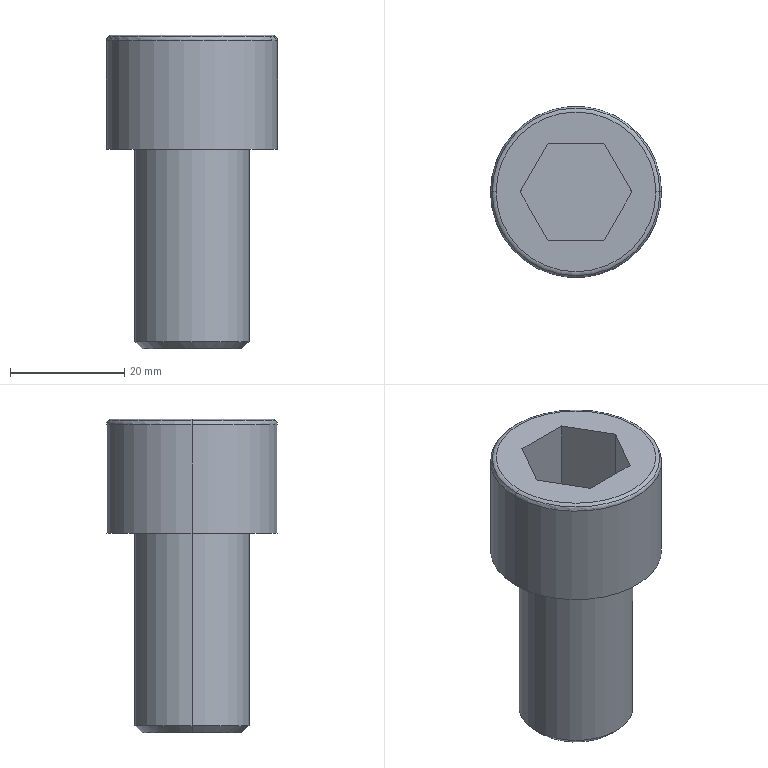Part | Creo | 1 solid | 20 faces | box 30 x 30 x 55 mm | volume 21762 mm3 | plane 10 | cylinder 4 | torus 4 | cone 2 | commonest cylinder face diameters 20 x2 30 x2
STEP:
#1=CARTESIAN_POINT('',(255.,70.,140.75));
#2=VERTEX_POINT('',#1);
#3=CARTESIAN_POINT('',(275.,70.,140.75));
#4=VERTEX_POINT('',#3);
#5=CARTESIAN_POINT('',(265.,70.,140.75));
#6=DIRECTION('',(0.,0.,-1.));
#7=DIRECTION('',(-1.,0.,0.));
#8=AXIS2_PLACEMENT_3D('',#5,#6,#7);
#9=CIRCLE('',#8,10.);
#10=EDGE_CURVE('',#2,#4,#9,.T.);
#11=ORIENTED_EDGE('',*,*,#10,.T.);
#12=CARTESIAN_POINT('',(275.,70.,174.5));
#13=VERTEX_POINT('',#12);
#14=CARTESIAN_POINT('',(275.,70.,174.5));
#15=DIRECTION('',(0.,0.,-1.));
#16=VECTOR('',#15,33.75);
#17=LINE('',#14,#16);
#18=EDGE_CURVE('',#13,#4,#17,.T.);
#19=ORIENTED_EDGE('',*,*,#18,.F.);
#20=CARTESIAN_POINT('',(255.,70.,174.5));
#21=VERTEX_POINT('',#20);
#22=CARTESIAN_POINT('',(265.,70.,174.5));
#23=DIRECTION('',(0.,0.,1.));
#24=DIRECTION('',(1.,0.,0.));
#25=AXIS2_PLACEMENT_3D('',#22,#23,#24);
#26=CIRCLE('',#25,10.);
#27=EDGE_CURVE('',#13,#21,#26,.T.);
#28=ORIENTED_EDGE('',*,*,#27,.T.);
#29=CARTESIAN_POINT('',(255.,70.,174.5));
#30=DIRECTION('',(0.,0.,-1.));
#31=VECTOR('',#30,33.75);
#32=LINE('',#29,#31);
#33=EDGE_CURVE('',#21,#2,#32,.T.);
#34=ORIENTED_EDGE('',*,*,#33,.T.);
#35=EDGE_LOOP('',(#11,#19,#28,#34));
#36=FACE_OUTER_BOUND('',#35,.F.);
#37=CARTESIAN_POINT('',(265.,70.,174.5));
#38=DIRECTION('',(0.,0.,-1.));
#39=DIRECTION('',(-1.,0.,0.));
#40=AXIS2_PLACEMENT_3D('',#37,#38,#39);
#41=CYLINDRICAL_SURFACE('',#40,10.);
#42=ADVANCED_FACE('',(#36),#41,.T.);
#43=CARTESIAN_POINT('',(256.25,70.,139.5));
#44=VERTEX_POINT('',#43);
#45=CARTESIAN_POINT('',(273.75,70.,139.5));
#46=VERTEX_POINT('',#45);
#47=CARTESIAN_POINT('',(265.,70.,139.5));
#48=DIRECTION('',(0.,0.,-1.));
#49=DIRECTION('',(-1.,0.,0.));
#50=AXIS2_PLACEMENT_3D('',#47,#48,#49);
#51=CIRCLE('',#50,8.75);
#52=EDGE_CURVE('',#44,#46,#51,.T.);
#53=ORIENTED_EDGE('',*,*,#52,.T.);
#54=CARTESIAN_POINT('',(273.75,70.,139.5));
#55=DIRECTION('',(0.7071,0.,0.7071));
#56=VECTOR('',#55,1.768);
#57=LINE('',#54,#56);
#58=EDGE_CURVE('',#46,#4,#57,.T.);
#59=ORIENTED_EDGE('',*,*,#58,.T.);
#60=ORIENTED_EDGE('',*,*,#10,.F.);
#61=CARTESIAN_POINT('',(256.25,70.,139.5));
#62=DIRECTION('',(-0.7071,0.,0.7071));
#63=VECTOR('',#62,1.768);
#64=LINE('',#61,#63);
#65=EDGE_CURVE('',#44,#2,#64,.T.);
#66=ORIENTED_EDGE('',*,*,#65,.F.);
#67=EDGE_LOOP('',(#53,#59,#60,#66));
#68=FACE_OUTER_BOUND('',#67,.F.);
#69=CARTESIAN_POINT('',(265.,70.,140.125));
#70=DIRECTION('',(0.,0.,1.));
#71=DIRECTION('',(1.,0.,0.));
#72=AXIS2_PLACEMENT_3D('',#69,#70,#71);
#73=CONICAL_SURFACE('',#72,9.375,45.);
#74=ADVANCED_FACE('',(#68),#73,.T.);
#75=CARTESIAN_POINT('',(265.,70.,139.5));
#76=DIRECTION('',(0.,0.,-1.));
#77=DIRECTION('',(1.,0.,0.));
#78=AXIS2_PLACEMENT_3D('',#75,#76,#77);
#79=CIRCLE('',#78,8.75);
#80=EDGE_CURVE('',#46,#44,#79,.T.);
#81=ORIENTED_EDGE('',*,*,#80,.F.);
#82=ORIENTED_EDGE('',*,*,#52,.F.);
#83=EDGE_LOOP('',(#81,#82));
#84=FACE_OUTER_BOUND('',#83,.F.);
#85=CARTESIAN_POINT('',(265.,70.,139.5));
#86=DIRECTION('',(0.,0.,1.));
#87=DIRECTION('',(1.,0.,0.));
#88=AXIS2_PLACEMENT_3D('',#85,#86,#87);
#89=PLANE('',#88);
#90=ADVANCED_FACE('',(#84),#89,.F.);
#91=ORIENTED_EDGE('',*,*,#80,.T.);
#92=ORIENTED_EDGE('',*,*,#65,.T.);
#93=CARTESIAN_POINT('',(265.,70.,140.75));
#94=DIRECTION('',(0.,0.,-1.));
#95=DIRECTION('',(1.,0.,0.));
#96=AXIS2_PLACEMENT_3D('',#93,#94,#95);
#97=CIRCLE('',#96,10.);
#98=EDGE_CURVE('',#4,#2,#97,.T.);
#99=ORIENTED_EDGE('',*,*,#98,.F.);
#100=ORIENTED_EDGE('',*,*,#58,.F.);
#101=EDGE_LOOP('',(#91,#92,#99,#100));
#102=FACE_OUTER_BOUND('',#101,.F.);
#103=CARTESIAN_POINT('',(265.,70.,140.125));
#104=DIRECTION('',(0.,0.,1.));
#105=DIRECTION('',(1.,0.,0.));
#106=AXIS2_PLACEMENT_3D('',#103,#104,#105);
#107=CONICAL_SURFACE('',#106,9.375,45.);
#108=ADVANCED_FACE('',(#102),#107,.T.);
#109=ORIENTED_EDGE('',*,*,#98,.T.);
#110=ORIENTED_EDGE('',*,*,#33,.F.);
#111=CARTESIAN_POINT('',(265.,70.,174.5));
#112=DIRECTION('',(0.,0.,1.));
#113=DIRECTION('',(-1.,0.,0.));
#114=AXIS2_PLACEMENT_3D('',#111,#112,#113);
#115=CIRCLE('',#114,10.);
#116=EDGE_CURVE('',#21,#13,#115,.T.);
#117=ORIENTED_EDGE('',*,*,#116,.T.);
#118=ORIENTED_EDGE('',*,*,#18,.T.);
#119=EDGE_LOOP('',(#109,#110,#117,#118));
#120=FACE_OUTER_BOUND('',#119,.F.);
#121=CARTESIAN_POINT('',(265.,70.,174.5));
#122=DIRECTION('',(0.,0.,-1.));
#123=DIRECTION('',(-1.,0.,0.));
#124=AXIS2_PLACEMENT_3D('',#121,#122,#123);
#125=CYLINDRICAL_SURFACE('',#124,10.);
#126=ADVANCED_FACE('',(#120),#125,.T.);
#127=CARTESIAN_POINT('',(280.,70.,174.5));
#128=VERTEX_POINT('',#127);
#129=CARTESIAN_POINT('',(250.,70.,174.5));
#130=VERTEX_POINT('',#129);
#131=CARTESIAN_POINT('',(265.,70.,174.5));
#132=DIRECTION('',(0.,0.,-1.));
#133=DIRECTION('',(1.,0.,0.));
#134=AXIS2_PLACEMENT_3D('',#131,#132,#133);
#135=CIRCLE('',#134,15.);
#136=EDGE_CURVE('',#128,#130,#135,.T.);
#137=ORIENTED_EDGE('',*,*,#136,.F.);
#138=CARTESIAN_POINT('',(265.,70.,174.5));
#139=DIRECTION('',(0.,0.,-1.));
#140=DIRECTION('',(-1.,0.,0.));
#141=AXIS2_PLACEMENT_3D('',#138,#139,#140);
#142=CIRCLE('',#141,15.);
#143=EDGE_CURVE('',#130,#128,#142,.T.);
#144=ORIENTED_EDGE('',*,*,#143,.F.);
#145=EDGE_LOOP('',(#137,#144));
#146=FACE_OUTER_BOUND('',#145,.F.);
#147=ORIENTED_EDGE('',*,*,#27,.F.);
#148=ORIENTED_EDGE('',*,*,#116,.F.);
#149=EDGE_LOOP('',(#147,#148));
#150=FACE_BOUND('',#149,.F.);
#151=CARTESIAN_POINT('',(265.,70.,174.5));
#152=DIRECTION('',(0.,0.,-1.));
#153=DIRECTION('',(-1.,0.,0.));
#154=AXIS2_PLACEMENT_3D('',#151,#152,#153);
#155=PLANE('',#154);
#156=ADVANCED_FACE('',(#146,#150),#155,.T.);
#157=CARTESIAN_POINT('',(250.,70.,193.5));
#158=VERTEX_POINT('',#157);
#159=CARTESIAN_POINT('',(280.,70.,193.5));
#160=VERTEX_POINT('',#159);
#161=CARTESIAN_POINT('',(265.,70.,193.5));
#162=DIRECTION('',(0.,0.,1.));
#163=DIRECTION('',(-1.,0.,0.));
#164=AXIS2_PLACEMENT_3D('',#161,#162,#163);
#165=CIRCLE('',#164,15.);
#166=EDGE_CURVE('',#158,#160,#165,.T.);
#167=ORIENTED_EDGE('',*,*,#166,.T.);
#168=CARTESIAN_POINT('',(280.,70.,174.5));
#169=DIRECTION('',(0.,0.,1.));
#170=VECTOR('',#169,19.);
#171=LINE('',#168,#170);
#172=EDGE_CURVE('',#128,#160,#171,.T.);
#173=ORIENTED_EDGE('',*,*,#172,.F.);
#174=ORIENTED_EDGE('',*,*,#136,.T.);
#175=CARTESIAN_POINT('',(250.,70.,174.5));
#176=DIRECTION('',(0.,0.,1.));
#177=VECTOR('',#176,19.);
#178=LINE('',#175,#177);
#179=EDGE_CURVE('',#130,#158,#178,.T.);
#180=ORIENTED_EDGE('',*,*,#179,.T.);
#181=EDGE_LOOP('',(#167,#173,#174,#180));
#182=FACE_OUTER_BOUND('',#181,.F.);
#183=CARTESIAN_POINT('',(265.,70.,174.5));
#184=DIRECTION('',(0.,0.,1.));
#185=DIRECTION('',(1.,0.,0.));
#186=AXIS2_PLACEMENT_3D('',#183,#184,#185);
#187=CYLINDRICAL_SURFACE('',#186,15.);
#188=ADVANCED_FACE('',(#182),#187,.T.);
#189=ORIENTED_EDGE('',*,*,#166,.F.);
#190=CARTESIAN_POINT('',(250.293,70.,194.207));
#191=VERTEX_POINT('',#190);
#192=CARTESIAN_POINT('',(251.,70.,193.5));
#193=DIRECTION('',(0.,1.,0.));
#194=DIRECTION('',(-1.,0.,0.));
#195=AXIS2_PLACEMENT_3D('',#192,#193,#194);
#196=CIRCLE('',#195,1.);
#197=EDGE_CURVE('',#158,#191,#196,.T.);
#198=ORIENTED_EDGE('',*,*,#197,.T.);
#199=CARTESIAN_POINT('',(279.707,70.,194.207));
#200=VERTEX_POINT('',#199);
#201=CARTESIAN_POINT('',(265.,70.,194.207));
#202=DIRECTION('',(0.,0.,1.));
#203=DIRECTION('',(-1.,0.,0.));
#204=AXIS2_PLACEMENT_3D('',#201,#202,#203);
#205=CIRCLE('',#204,14.707);
#206=EDGE_CURVE('',#191,#200,#205,.T.);
#207=ORIENTED_EDGE('',*,*,#206,.T.);
#208=CARTESIAN_POINT('',(279.,70.,193.5));
#209=DIRECTION('',(0.,-1.,0.));
#210=DIRECTION('',(1.,0.,0.));
#211=AXIS2_PLACEMENT_3D('',#208,#209,#210);
#212=CIRCLE('',#211,1.);
#213=EDGE_CURVE('',#160,#200,#212,.T.);
#214=ORIENTED_EDGE('',*,*,#213,.F.);
#215=EDGE_LOOP('',(#189,#198,#207,#214));
#216=FACE_OUTER_BOUND('',#215,.F.);
#217=CARTESIAN_POINT('',(265.,70.,193.5));
#218=DIRECTION('',(0.,0.,1.));
#219=DIRECTION('',(1.,0.,0.));
#220=AXIS2_PLACEMENT_3D('',#217,#218,#219);
#221=TOROIDAL_SURFACE('',#220,14.,1.);
#222=ADVANCED_FACE('',(#216),#221,.T.);
#223=CARTESIAN_POINT('',(265.,70.,193.5));
#224=DIRECTION('',(0.,0.,1.));
#225=DIRECTION('',(1.,0.,0.));
#226=AXIS2_PLACEMENT_3D('',#223,#224,#225);
#227=CIRCLE('',#226,15.);
#228=EDGE_CURVE('',#160,#158,#227,.T.);
#229=ORIENTED_EDGE('',*,*,#228,.F.);
#230=ORIENTED_EDGE('',*,*,#213,.T.);
#231=CARTESIAN_POINT('',(265.,70.,194.207));
#232=DIRECTION('',(0.,0.,1.));
#233=DIRECTION('',(1.,0.,0.));
#234=AXIS2_PLACEMENT_3D('',#231,#232,#233);
#235=CIRCLE('',#234,14.707);
#236=EDGE_CURVE('',#200,#191,#235,.T.);
#237=ORIENTED_EDGE('',*,*,#236,.T.);
#238=ORIENTED_EDGE('',*,*,#197,.F.);
#239=EDGE_LOOP('',(#229,#230,#237,#238));
#240=FACE_OUTER_BOUND('',#239,.F.);
#241=CARTESIAN_POINT('',(265.,70.,193.5));
#242=DIRECTION('',(0.,0.,1.));
#243=DIRECTION('',(1.,0.,0.));
#244=AXIS2_PLACEMENT_3D('',#241,#242,#243);
#245=TOROIDAL_SURFACE('',#244,14.,1.);
#246=ADVANCED_FACE('',(#240),#245,.T.);
#247=ORIENTED_EDGE('',*,*,#228,.T.);
#248=ORIENTED_EDGE('',*,*,#179,.F.);
#249=ORIENTED_EDGE('',*,*,#143,.T.);
#250=ORIENTED_EDGE('',*,*,#172,.T.);
#251=EDGE_LOOP('',(#247,#248,#249,#250));
#252=FACE_OUTER_BOUND('',#251,.F.);
#253=CARTESIAN_POINT('',(265.,70.,174.5));
#254=DIRECTION('',(0.,0.,1.));
#255=DIRECTION('',(1.,0.,0.));
#256=AXIS2_PLACEMENT_3D('',#253,#254,#255);
#257=CYLINDRICAL_SURFACE('',#256,15.);
#258=ADVANCED_FACE('',(#252),#257,.T.);
#259=CARTESIAN_POINT('',(279.,70.,194.5));
#260=VERTEX_POINT('',#259);
#261=CARTESIAN_POINT('',(251.,70.,194.5));
#262=VERTEX_POINT('',#261);
#263=CARTESIAN_POINT('',(265.,70.,194.5));
#264=DIRECTION('',(0.,0.,1.));
#265=DIRECTION('',(1.,0.,0.));
#266=AXIS2_PLACEMENT_3D('',#263,#264,#265);
#267=CIRCLE('',#266,14.);
#268=EDGE_CURVE('',#260,#262,#267,.T.);
#269=ORIENTED_EDGE('',*,*,#268,.T.);
#270=CARTESIAN_POINT('',(251.,70.,193.5));
#271=DIRECTION('',(0.,1.,0.));
#272=DIRECTION('',(-0.7071,0.,0.7071));
#273=AXIS2_PLACEMENT_3D('',#270,#271,#272);
#274=CIRCLE('',#273,1.);
#275=EDGE_CURVE('',#191,#262,#274,.T.);
#276=ORIENTED_EDGE('',*,*,#275,.F.);
#277=ORIENTED_EDGE('',*,*,#236,.F.);
#278=CARTESIAN_POINT('',(279.,70.,193.5));
#279=DIRECTION('',(0.,-1.,0.));
#280=DIRECTION('',(0.7071,0.,0.7071));
#281=AXIS2_PLACEMENT_3D('',#278,#279,#280);
#282=CIRCLE('',#281,1.);
#283=EDGE_CURVE('',#200,#260,#282,.T.);
#284=ORIENTED_EDGE('',*,*,#283,.T.);
#285=EDGE_LOOP('',(#269,#276,#277,#284));
#286=FACE_OUTER_BOUND('',#285,.F.);
#287=CARTESIAN_POINT('',(265.,70.,193.5));
#288=DIRECTION('',(0.,0.,1.));
#289=DIRECTION('',(1.,0.,0.));
#290=AXIS2_PLACEMENT_3D('',#287,#288,#289);
#291=TOROIDAL_SURFACE('',#290,14.,1.);
#292=ADVANCED_FACE('',(#286),#291,.T.);
#293=ORIENTED_EDGE('',*,*,#268,.F.);
#294=CARTESIAN_POINT('',(265.,70.,194.5));
#295=DIRECTION('',(0.,0.,1.));
#296=DIRECTION('',(-1.,0.,0.));
#297=AXIS2_PLACEMENT_3D('',#294,#295,#296);
#298=CIRCLE('',#297,14.);
#299=EDGE_CURVE('',#262,#260,#298,.T.);
#300=ORIENTED_EDGE('',*,*,#299,.F.);
#301=EDGE_LOOP('',(#293,#300));
#302=FACE_OUTER_BOUND('',#301,.F.);
#303=CARTESIAN_POINT('',(269.907,61.5,194.5));
#304=VERTEX_POINT('',#303);
#305=CARTESIAN_POINT('',(260.093,61.5,194.5));
#306=VERTEX_POINT('',#305);
#307=CARTESIAN_POINT('',(269.907,61.5,194.5));
#308=DIRECTION('',(-1.,0.,0.));
#309=VECTOR('',#308,9.815);
#310=LINE('',#307,#309);
#311=EDGE_CURVE('',#304,#306,#310,.T.);
#312=ORIENTED_EDGE('',*,*,#311,.F.);
#313=CARTESIAN_POINT('',(274.815,70.,194.5));
#314=VERTEX_POINT('',#313);
#315=CARTESIAN_POINT('',(274.815,70.,194.5));
#316=DIRECTION('',(-0.5,-0.866,0.));
#317=VECTOR('',#316,9.815);
#318=LINE('',#315,#317);
#319=EDGE_CURVE('',#314,#304,#318,.T.);
#320=ORIENTED_EDGE('',*,*,#319,.F.);
#321=CARTESIAN_POINT('',(269.907,78.5,194.5));
#322=VERTEX_POINT('',#321);
#323=CARTESIAN_POINT('',(269.907,78.5,194.5));
#324=DIRECTION('',(0.5,-0.866,0.));
#325=VECTOR('',#324,9.815);
#326=LINE('',#323,#325);
#327=EDGE_CURVE('',#322,#314,#326,.T.);
#328=ORIENTED_EDGE('',*,*,#327,.F.);
#329=CARTESIAN_POINT('',(260.093,78.5,194.5));
#330=VERTEX_POINT('',#329);
#331=CARTESIAN_POINT('',(260.093,78.5,194.5));
#332=DIRECTION('',(1.,0.,0.));
#333=VECTOR('',#332,9.815);
#334=LINE('',#331,#333);
#335=EDGE_CURVE('',#330,#322,#334,.T.);
#336=ORIENTED_EDGE('',*,*,#335,.F.);
#337=CARTESIAN_POINT('',(255.185,70.,194.5));
#338=VERTEX_POINT('',#337);
#339=CARTESIAN_POINT('',(255.185,70.,194.5));
#340=DIRECTION('',(0.5,0.866,0.));
#341=VECTOR('',#340,9.815);
#342=LINE('',#339,#341);
#343=EDGE_CURVE('',#338,#330,#342,.T.);
#344=ORIENTED_EDGE('',*,*,#343,.F.);
#345=CARTESIAN_POINT('',(260.093,61.5,194.5));
#346=DIRECTION('',(-0.5,0.866,0.));
#347=VECTOR('',#346,9.815);
#348=LINE('',#345,#347);
#349=EDGE_CURVE('',#306,#338,#348,.T.);
#350=ORIENTED_EDGE('',*,*,#349,.F.);
#351=EDGE_LOOP('',(#312,#320,#328,#336,#344,#350));
#352=FACE_BOUND('',#351,.F.);
#353=CARTESIAN_POINT('',(265.,70.,194.5));
#354=DIRECTION('',(0.,0.,1.));
#355=DIRECTION('',(1.,0.,0.));
#356=AXIS2_PLACEMENT_3D('',#353,#354,#355);
#357=PLANE('',#356);
#358=ADVANCED_FACE('',(#302,#352),#357,.T.);
#359=ORIENTED_EDGE('',*,*,#299,.T.);
#360=ORIENTED_EDGE('',*,*,#283,.F.);
#361=ORIENTED_EDGE('',*,*,#206,.F.);
#362=ORIENTED_EDGE('',*,*,#275,.T.);
#363=EDGE_LOOP('',(#359,#360,#361,#362));
#364=FACE_OUTER_BOUND('',#363,.F.);
#365=CARTESIAN_POINT('',(265.,70.,193.5));
#366=DIRECTION('',(0.,0.,1.));
#367=DIRECTION('',(1.,0.,0.));
#368=AXIS2_PLACEMENT_3D('',#365,#366,#367);
#369=TOROIDAL_SURFACE('',#368,14.,1.);
#370=ADVANCED_FACE('',(#364),#369,.T.);
#371=ORIENTED_EDGE('',*,*,#311,.T.);
#372=CARTESIAN_POINT('',(260.093,61.5,181.3));
#373=VERTEX_POINT('',#372);
#374=CARTESIAN_POINT('',(260.093,61.5,194.5));
#375=DIRECTION('',(0.,0.,-1.));
#376=VECTOR('',#375,13.2);
#377=LINE('',#374,#376);
#378=EDGE_CURVE('',#306,#373,#377,.T.);
#379=ORIENTED_EDGE('',*,*,#378,.T.);
#380=CARTESIAN_POINT('',(269.907,61.5,181.3));
#381=VERTEX_POINT('',#380);
#382=CARTESIAN_POINT('',(269.907,61.5,181.3));
#383=DIRECTION('',(-1.,0.,0.));
#384=VECTOR('',#383,9.815);
#385=LINE('',#382,#384);
#386=EDGE_CURVE('',#381,#373,#385,.T.);
#387=ORIENTED_EDGE('',*,*,#386,.F.);
#388=CARTESIAN_POINT('',(269.907,61.5,194.5));
#389=DIRECTION('',(0.,0.,-1.));
#390=VECTOR('',#389,13.2);
#391=LINE('',#388,#390);
#392=EDGE_CURVE('',#304,#381,#391,.T.);
#393=ORIENTED_EDGE('',*,*,#392,.F.);
#394=EDGE_LOOP('',(#371,#379,#387,#393));
#395=FACE_OUTER_BOUND('',#394,.F.);
#396=CARTESIAN_POINT('',(260.093,61.5,181.3));
#397=DIRECTION('',(0.,-1.,0.));
#398=DIRECTION('',(0.,0.,-1.));
#399=AXIS2_PLACEMENT_3D('',#396,#397,#398);
#400=PLANE('',#399);
#401=ADVANCED_FACE('',(#395),#400,.F.);
#402=ORIENTED_EDGE('',*,*,#349,.T.);
#403=CARTESIAN_POINT('',(255.185,70.,181.3));
#404=VERTEX_POINT('',#403);
#405=CARTESIAN_POINT('',(255.185,70.,194.5));
#406=DIRECTION('',(0.,0.,-1.));
#407=VECTOR('',#406,13.2);
#408=LINE('',#405,#407);
#409=EDGE_CURVE('',#338,#404,#408,.T.);
#410=ORIENTED_EDGE('',*,*,#409,.T.);
#411=CARTESIAN_POINT('',(255.185,70.,181.3));
#412=DIRECTION('',(0.5,-0.866,0.));
#413=VECTOR('',#412,9.815);
#414=LINE('',#411,#413);
#415=EDGE_CURVE('',#404,#373,#414,.T.);
#416=ORIENTED_EDGE('',*,*,#415,.T.);
#417=ORIENTED_EDGE('',*,*,#378,.F.);
#418=EDGE_LOOP('',(#402,#410,#416,#417));
#419=FACE_OUTER_BOUND('',#418,.F.);
#420=CARTESIAN_POINT('',(255.185,70.,181.3));
#421=DIRECTION('',(-0.866,-0.5,0.));
#422=DIRECTION('',(0.5,-0.866,0.));
#423=AXIS2_PLACEMENT_3D('',#420,#421,#422);
#424=PLANE('',#423);
#425=ADVANCED_FACE('',(#419),#424,.F.);
#426=ORIENTED_EDGE('',*,*,#343,.T.);
#427=CARTESIAN_POINT('',(260.093,78.5,181.3));
#428=VERTEX_POINT('',#427);
#429=CARTESIAN_POINT('',(260.093,78.5,194.5));
#430=DIRECTION('',(0.,0.,-1.));
#431=VECTOR('',#430,13.2);
#432=LINE('',#429,#431);
#433=EDGE_CURVE('',#330,#428,#432,.T.);
#434=ORIENTED_EDGE('',*,*,#433,.T.);
#435=CARTESIAN_POINT('',(260.093,78.5,181.3));
#436=DIRECTION('',(-0.5,-0.866,0.));
#437=VECTOR('',#436,9.815);
#438=LINE('',#435,#437);
#439=EDGE_CURVE('',#428,#404,#438,.T.);
#440=ORIENTED_EDGE('',*,*,#439,.T.);
#441=ORIENTED_EDGE('',*,*,#409,.F.);
#442=EDGE_LOOP('',(#426,#434,#440,#441));
#443=FACE_OUTER_BOUND('',#442,.F.);
#444=CARTESIAN_POINT('',(260.093,78.5,181.3));
#445=DIRECTION('',(-0.866,0.5,0.));
#446=DIRECTION('',(-0.5,-0.866,0.));
#447=AXIS2_PLACEMENT_3D('',#444,#445,#446);
#448=PLANE('',#447);
#449=ADVANCED_FACE('',(#443),#448,.F.);
#450=ORIENTED_EDGE('',*,*,#335,.T.);
#451=CARTESIAN_POINT('',(269.907,78.5,181.3));
#452=VERTEX_POINT('',#451);
#453=CARTESIAN_POINT('',(269.907,78.5,194.5));
#454=DIRECTION('',(0.,0.,-1.));
#455=VECTOR('',#454,13.2);
#456=LINE('',#453,#455);
#457=EDGE_CURVE('',#322,#452,#456,.T.);
#458=ORIENTED_EDGE('',*,*,#457,.T.);
#459=CARTESIAN_POINT('',(260.093,78.5,181.3));
#460=DIRECTION('',(1.,0.,0.));
#461=VECTOR('',#460,9.815);
#462=LINE('',#459,#461);
#463=EDGE_CURVE('',#428,#452,#462,.T.);
#464=ORIENTED_EDGE('',*,*,#463,.F.);
#465=ORIENTED_EDGE('',*,*,#433,.F.);
#466=EDGE_LOOP('',(#450,#458,#464,#465));
#467=FACE_OUTER_BOUND('',#466,.F.);
#468=CARTESIAN_POINT('',(269.907,78.5,181.3));
#469=DIRECTION('',(0.,1.,0.));
#470=DIRECTION('',(0.,0.,1.));
#471=AXIS2_PLACEMENT_3D('',#468,#469,#470);
#472=PLANE('',#471);
#473=ADVANCED_FACE('',(#467),#472,.F.);
#474=ORIENTED_EDGE('',*,*,#327,.T.);
#475=CARTESIAN_POINT('',(274.815,70.,181.3));
#476=VERTEX_POINT('',#475);
#477=CARTESIAN_POINT('',(274.815,70.,194.5));
#478=DIRECTION('',(0.,0.,-1.));
#479=VECTOR('',#478,13.2);
#480=LINE('',#477,#479);
#481=EDGE_CURVE('',#314,#476,#480,.T.);
#482=ORIENTED_EDGE('',*,*,#481,.T.);
#483=CARTESIAN_POINT('',(274.815,70.,181.3));
#484=DIRECTION('',(-0.5,0.866,0.));
#485=VECTOR('',#484,9.815);
#486=LINE('',#483,#485);
#487=EDGE_CURVE('',#476,#452,#486,.T.);
#488=ORIENTED_EDGE('',*,*,#487,.T.);
#489=ORIENTED_EDGE('',*,*,#457,.F.);
#490=EDGE_LOOP('',(#474,#482,#488,#489));
#491=FACE_OUTER_BOUND('',#490,.F.);
#492=CARTESIAN_POINT('',(274.815,70.,181.3));
#493=DIRECTION('',(0.866,0.5,0.));
#494=DIRECTION('',(-0.5,0.866,0.));
#495=AXIS2_PLACEMENT_3D('',#492,#493,#494);
#496=PLANE('',#495);
#497=ADVANCED_FACE('',(#491),#496,.F.);
#498=ORIENTED_EDGE('',*,*,#319,.T.);
#499=ORIENTED_EDGE('',*,*,#392,.T.);
#500=CARTESIAN_POINT('',(269.907,61.5,181.3));
#501=DIRECTION('',(0.5,0.866,0.));
#502=VECTOR('',#501,9.815);
#503=LINE('',#500,#502);
#504=EDGE_CURVE('',#381,#476,#503,.T.);
#505=ORIENTED_EDGE('',*,*,#504,.T.);
#506=ORIENTED_EDGE('',*,*,#481,.F.);
#507=EDGE_LOOP('',(#498,#499,#505,#506));
#508=FACE_OUTER_BOUND('',#507,.F.);
#509=CARTESIAN_POINT('',(269.907,61.5,181.3));
#510=DIRECTION('',(0.866,-0.5,0.));
#511=DIRECTION('',(0.5,0.866,0.));
#512=AXIS2_PLACEMENT_3D('',#509,#510,#511);
#513=PLANE('',#512);
#514=ADVANCED_FACE('',(#508),#513,.F.);
#515=ORIENTED_EDGE('',*,*,#386,.T.);
#516=ORIENTED_EDGE('',*,*,#415,.F.);
#517=ORIENTED_EDGE('',*,*,#439,.F.);
#518=ORIENTED_EDGE('',*,*,#463,.T.);
#519=ORIENTED_EDGE('',*,*,#487,.F.);
#520=ORIENTED_EDGE('',*,*,#504,.F.);
#521=EDGE_LOOP('',(#515,#516,#517,#518,#519,#520));
#522=FACE_OUTER_BOUND('',#521,.F.);
#523=CARTESIAN_POINT('',(269.907,61.5,181.3));
#524=DIRECTION('',(0.,0.,1.));
#525=DIRECTION('',(1.,0.,0.));
#526=AXIS2_PLACEMENT_3D('',#523,#524,#525);
#527=PLANE('',#526);
#528=ADVANCED_FACE('',(#522),#527,.T.);
#529=CLOSED_SHELL('',(#42,#74,#90,#108,#126,#156,#188,#222,#246,#258,#292,#358,#370,#401,#425,#449,#473,#497,#514,#528));
#530=MANIFOLD_SOLID_BREP('',#529);
#531=(LENGTH_UNIT()NAMED_UNIT(*)SI_UNIT(.MILLI.,.METRE.));
#532=UNCERTAINTY_MEASURE_WITH_UNIT(LENGTH_MEASURE(0.006947),#531,'','');
#533=(NAMED_UNIT(*)PLANE_ANGLE_UNIT()SI_UNIT($,.RADIAN.));
#534=PLANE_ANGLE_MEASURE_WITH_UNIT(PLANE_ANGLE_MEASURE(0.01745),#533);
#535=(CONVERSION_BASED_UNIT('DEGREE',#534)NAMED_UNIT(*)PLANE_ANGLE_UNIT());
#536=(NAMED_UNIT(*)SI_UNIT($,.STERADIAN.)SOLID_ANGLE_UNIT());
#537=(GEOMETRIC_REPRESENTATION_CONTEXT(3)GLOBAL_UNCERTAINTY_ASSIGNED_CONTEXT((#532))GLOBAL_UNIT_ASSIGNED_CONTEXT((#531,#535,#536))REPRESENTATION_CONTEXT('',''));
#538=ADVANCED_BREP_SHAPE_REPRESENTATION('',(#530),#537);